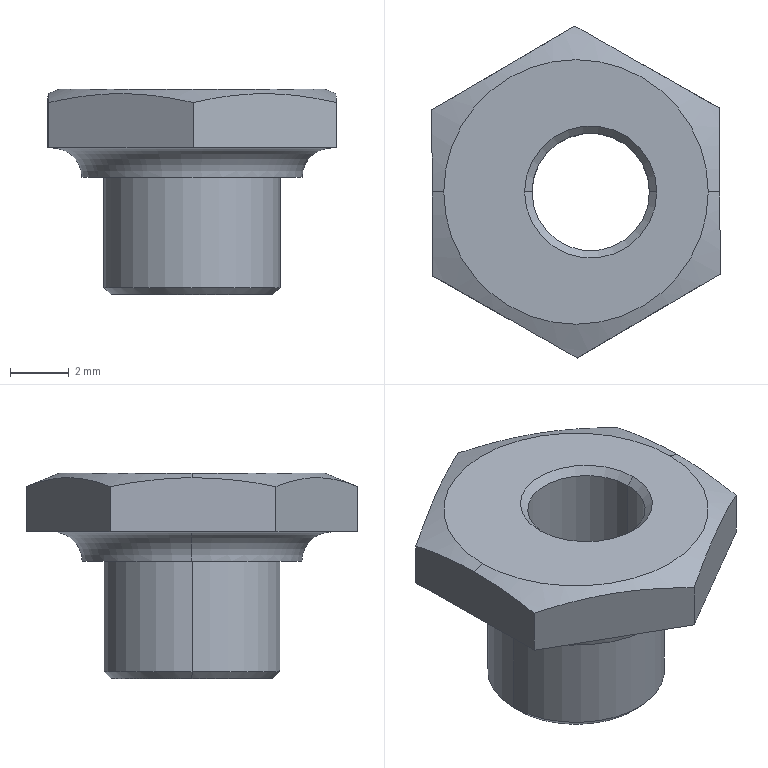Part | NX | features BREP 1 | 1 solid | 24 faces | box 9.818 x 11.293 x 7 mm | volume 236.126 mm3 | plane 10 | cone 8 | cylinder 4 | torus 2 | commonest cylinder face diameters 4 x2 6 x2
STEP:
#1=CARTESIAN_POINT('',(-3.,0.,0.25));
#2=VERTEX_POINT('',#1);
#3=CARTESIAN_POINT('',(-2.75,0.,0.));
#4=VERTEX_POINT('',#3);
#5=CARTESIAN_POINT('',(-3.,0.,0.25));
#6=DIRECTION('',(-0.7071,0.,0.7071));
#7=VECTOR('',#6,1000.);
#8=LINE('',#5,#7);
#9=EDGE_CURVE('',#2,#4,#8,.F.);
#10=ORIENTED_EDGE('',*,*,#9,.T.);
#11=CARTESIAN_POINT('',(2.75,0.,0.));
#12=VERTEX_POINT('',#11);
#13=CARTESIAN_POINT('',(0.,0.,0.));
#14=DIRECTION('',(0.,0.,-1.));
#15=DIRECTION('',(1.,0.,0.));
#16=AXIS2_PLACEMENT_3D('',#13,#14,#15);
#17=CIRCLE('',#16,2.75);
#18=EDGE_CURVE('',#12,#4,#17,.T.);
#19=ORIENTED_EDGE('',*,*,#18,.F.);
#20=CARTESIAN_POINT('',(3.,0.,0.25));
#21=VERTEX_POINT('',#20);
#22=CARTESIAN_POINT('',(3.,0.,0.25));
#23=DIRECTION('',(0.7071,0.,0.7071));
#24=VECTOR('',#23,1000.);
#25=LINE('',#22,#24);
#26=EDGE_CURVE('',#21,#12,#25,.F.);
#27=ORIENTED_EDGE('',*,*,#26,.F.);
#28=CARTESIAN_POINT('',(0.,0.,0.25));
#29=DIRECTION('',(0.,0.,1.));
#30=DIRECTION('',(1.,0.,0.));
#31=AXIS2_PLACEMENT_3D('',#28,#29,#30);
#32=CIRCLE('',#31,3.);
#33=EDGE_CURVE('',#2,#21,#32,.T.);
#34=ORIENTED_EDGE('',*,*,#33,.F.);
#35=EDGE_LOOP('',(#10,#19,#27,#34));
#36=FACE_BOUND('',#35,.T.);
#37=CARTESIAN_POINT('',(0.,0.,0.25));
#38=DIRECTION('',(0.,0.,1.));
#39=DIRECTION('',(1.,0.,0.));
#40=AXIS2_PLACEMENT_3D('',#37,#38,#39);
#41=CONICAL_SURFACE('',#40,3.,0.7854);
#42=ADVANCED_FACE('',(#36),#41,.T.);
#43=CARTESIAN_POINT('',(2.5,0.,0.25));
#44=VERTEX_POINT('',#43);
#45=CARTESIAN_POINT('',(2.75,0.,0.));
#46=DIRECTION('',(0.7071,0.,-0.7071));
#47=VECTOR('',#46,1000.);
#48=LINE('',#45,#47);
#49=EDGE_CURVE('',#44,#12,#48,.T.);
#50=ORIENTED_EDGE('',*,*,#49,.F.);
#51=CARTESIAN_POINT('',(-1.5,0.,0.25));
#52=VERTEX_POINT('',#51);
#53=CARTESIAN_POINT('',(0.5,0.,0.25));
#54=DIRECTION('',(0.,0.,-1.));
#55=DIRECTION('',(1.,0.,0.));
#56=AXIS2_PLACEMENT_3D('',#53,#54,#55);
#57=CIRCLE('',#56,2.);
#58=EDGE_CURVE('',#52,#44,#57,.T.);
#59=ORIENTED_EDGE('',*,*,#58,.F.);
#60=CARTESIAN_POINT('',(-1.75,0.,0.));
#61=VERTEX_POINT('',#60);
#62=CARTESIAN_POINT('',(-1.75,0.,0.));
#63=DIRECTION('',(-0.7071,0.,-0.7071));
#64=VECTOR('',#63,1000.);
#65=LINE('',#62,#64);
#66=EDGE_CURVE('',#52,#61,#65,.T.);
#67=ORIENTED_EDGE('',*,*,#66,.T.);
#68=CARTESIAN_POINT('',(0.5,0.,0.));
#69=DIRECTION('',(0.,0.,1.));
#70=DIRECTION('',(1.,0.,0.));
#71=AXIS2_PLACEMENT_3D('',#68,#69,#70);
#72=CIRCLE('',#71,2.25);
#73=EDGE_CURVE('',#12,#61,#72,.T.);
#74=ORIENTED_EDGE('',*,*,#73,.F.);
#75=EDGE_LOOP('',(#50,#59,#67,#74));
#76=FACE_BOUND('',#75,.T.);
#77=CARTESIAN_POINT('',(0.5,0.,0.));
#78=DIRECTION('',(0.,0.,-1.));
#79=DIRECTION('',(-1.,0.,0.));
#80=AXIS2_PLACEMENT_3D('',#77,#78,#79);
#81=CONICAL_SURFACE('',#80,2.25,0.7854);
#82=ADVANCED_FACE('',(#76),#81,.F.);
#83=CARTESIAN_POINT('',(-1.75,0.,7.));
#84=VERTEX_POINT('',#83);
#85=CARTESIAN_POINT('',(-1.5,0.,6.75));
#86=VERTEX_POINT('',#85);
#87=CARTESIAN_POINT('',(-1.5,0.,6.75));
#88=DIRECTION('',(-0.7071,0.,0.7071));
#89=VECTOR('',#88,1000.);
#90=LINE('',#87,#89);
#91=EDGE_CURVE('',#84,#86,#90,.F.);
#92=ORIENTED_EDGE('',*,*,#91,.T.);
#93=CARTESIAN_POINT('',(2.5,0.,6.75));
#94=VERTEX_POINT('',#93);
#95=CARTESIAN_POINT('',(0.5,0.,6.75));
#96=DIRECTION('',(0.,0.,1.));
#97=DIRECTION('',(1.,0.,0.));
#98=AXIS2_PLACEMENT_3D('',#95,#96,#97);
#99=CIRCLE('',#98,2.);
#100=EDGE_CURVE('',#94,#86,#99,.T.);
#101=ORIENTED_EDGE('',*,*,#100,.F.);
#102=CARTESIAN_POINT('',(2.75,0.,7.));
#103=VERTEX_POINT('',#102);
#104=CARTESIAN_POINT('',(2.5,0.,6.75));
#105=DIRECTION('',(0.7071,0.,0.7071));
#106=VECTOR('',#105,1000.);
#107=LINE('',#104,#106);
#108=EDGE_CURVE('',#103,#94,#107,.F.);
#109=ORIENTED_EDGE('',*,*,#108,.F.);
#110=CARTESIAN_POINT('',(0.5,0.,7.));
#111=DIRECTION('',(0.,0.,-1.));
#112=DIRECTION('',(1.,0.,0.));
#113=AXIS2_PLACEMENT_3D('',#110,#111,#112);
#114=CIRCLE('',#113,2.25);
#115=EDGE_CURVE('',#84,#103,#114,.T.);
#116=ORIENTED_EDGE('',*,*,#115,.F.);
#117=EDGE_LOOP('',(#92,#101,#109,#116));
#118=FACE_BOUND('',#117,.T.);
#119=CARTESIAN_POINT('',(0.5,0.,6.75));
#120=DIRECTION('',(0.,0.,1.));
#121=DIRECTION('',(1.,0.,0.));
#122=AXIS2_PLACEMENT_3D('',#119,#120,#121);
#123=CONICAL_SURFACE('',#122,2.,0.7854);
#124=ADVANCED_FACE('',(#118),#123,.F.);
#125=CARTESIAN_POINT('',(-3.75,0.,4.));
#126=VERTEX_POINT('',#125);
#127=CARTESIAN_POINT('',(-4.75,0.,5.));
#128=VERTEX_POINT('',#127);
#129=CARTESIAN_POINT('',(-4.75,0.,4.));
#130=DIRECTION('',(0.,1.,0.));
#131=DIRECTION('',(-1.,0.,0.));
#132=AXIS2_PLACEMENT_3D('',#129,#130,#131);
#133=CIRCLE('',#132,1.);
#134=EDGE_CURVE('',#126,#128,#133,.F.);
#135=ORIENTED_EDGE('',*,*,#134,.T.);
#136=CARTESIAN_POINT('',(4.75,0.,5.));
#137=VERTEX_POINT('',#136);
#138=CARTESIAN_POINT('',(0.,0.,5.));
#139=DIRECTION('',(0.,0.,1.));
#140=DIRECTION('',(1.,0.,0.));
#141=AXIS2_PLACEMENT_3D('',#138,#139,#140);
#142=CIRCLE('',#141,4.75);
#143=EDGE_CURVE('',#137,#128,#142,.T.);
#144=ORIENTED_EDGE('',*,*,#143,.F.);
#145=CARTESIAN_POINT('',(3.75,0.,4.));
#146=VERTEX_POINT('',#145);
#147=CARTESIAN_POINT('',(4.75,0.,4.));
#148=DIRECTION('',(0.,-1.,0.));
#149=DIRECTION('',(0.,0.,-1.));
#150=AXIS2_PLACEMENT_3D('',#147,#148,#149);
#151=CIRCLE('',#150,1.);
#152=EDGE_CURVE('',#146,#137,#151,.F.);
#153=ORIENTED_EDGE('',*,*,#152,.F.);
#154=CARTESIAN_POINT('',(0.,0.,4.));
#155=DIRECTION('',(0.,0.,-1.));
#156=DIRECTION('',(-1.,0.,0.));
#157=AXIS2_PLACEMENT_3D('',#154,#155,#156);
#158=CIRCLE('',#157,3.75);
#159=EDGE_CURVE('',#126,#146,#158,.T.);
#160=ORIENTED_EDGE('',*,*,#159,.F.);
#161=EDGE_LOOP('',(#135,#144,#153,#160));
#162=FACE_BOUND('',#161,.T.);
#163=CARTESIAN_POINT('',(0.,0.,4.));
#164=DIRECTION('',(0.,0.,1.));
#165=DIRECTION('',(1.,0.,0.));
#166=AXIS2_PLACEMENT_3D('',#163,#164,#165);
#167=TOROIDAL_SURFACE('',#166,4.75,1.);
#168=ADVANCED_FACE('',(#162),#167,.F.);
#169=CARTESIAN_POINT('',(-3.,0.,4.));
#170=VERTEX_POINT('',#169);
#171=CARTESIAN_POINT('',(3.,0.,4.));
#172=VERTEX_POINT('',#171);
#173=CARTESIAN_POINT('',(0.,0.,4.));
#174=DIRECTION('',(0.,0.,-1.));
#175=DIRECTION('',(-1.,0.,0.));
#176=AXIS2_PLACEMENT_3D('',#173,#174,#175);
#177=CIRCLE('',#176,3.);
#178=EDGE_CURVE('',#170,#172,#177,.T.);
#179=ORIENTED_EDGE('',*,*,#178,.F.);
#180=CARTESIAN_POINT('',(0.,0.,4.));
#181=DIRECTION('',(0.,0.,-1.));
#182=DIRECTION('',(-1.,0.,0.));
#183=AXIS2_PLACEMENT_3D('',#180,#181,#182);
#184=CIRCLE('',#183,3.);
#185=EDGE_CURVE('',#172,#170,#184,.T.);
#186=ORIENTED_EDGE('',*,*,#185,.F.);
#187=EDGE_LOOP('',(#179,#186));
#188=FACE_BOUND('',#187,.T.);
#189=CARTESIAN_POINT('',(0.,0.,4.));
#190=DIRECTION('',(0.,0.,-1.));
#191=DIRECTION('',(-1.,0.,0.));
#192=AXIS2_PLACEMENT_3D('',#189,#190,#191);
#193=CIRCLE('',#192,3.75);
#194=EDGE_CURVE('',#146,#126,#193,.T.);
#195=ORIENTED_EDGE('',*,*,#194,.T.);
#196=ORIENTED_EDGE('',*,*,#159,.T.);
#197=EDGE_LOOP('',(#195,#196));
#198=FACE_BOUND('',#197,.T.);
#199=CARTESIAN_POINT('',(0.,0.,4.));
#200=DIRECTION('',(0.,0.,-1.));
#201=DIRECTION('',(-1.,0.,0.));
#202=AXIS2_PLACEMENT_3D('',#199,#200,#201);
#203=PLANE('',#202);
#204=ADVANCED_FACE('',(#188,#198),#203,.T.);
#205=CARTESIAN_POINT('',(-4.909,2.79,5.));
#206=VERTEX_POINT('',#205);
#207=CARTESIAN_POINT('',(-4.909,2.79,6.541));
#208=VERTEX_POINT('',#207);
#209=CARTESIAN_POINT('',(-4.909,2.79,5.));
#210=DIRECTION('',(0.,0.,1.));
#211=VECTOR('',#210,1000.);
#212=LINE('',#209,#211);
#213=EDGE_CURVE('',#206,#208,#212,.T.);
#214=ORIENTED_EDGE('',*,*,#213,.F.);
#215=CARTESIAN_POINT('',(-4.871,-2.857,5.));
#216=VERTEX_POINT('',#215);
#217=CARTESIAN_POINT('',(-4.909,2.79,5.));
#218=DIRECTION('',(0.006849,-1.,0.));
#219=VECTOR('',#218,1000.);
#220=LINE('',#217,#219);
#221=EDGE_CURVE('',#206,#216,#220,.T.);
#222=ORIENTED_EDGE('',*,*,#221,.T.);
#223=CARTESIAN_POINT('',(-4.871,-2.857,6.541));
#224=VERTEX_POINT('',#223);
#225=CARTESIAN_POINT('',(-4.871,-2.857,5.));
#226=DIRECTION('',(0.,0.,1.));
#227=VECTOR('',#226,1000.);
#228=LINE('',#225,#227);
#229=EDGE_CURVE('',#216,#224,#228,.T.);
#230=ORIENTED_EDGE('',*,*,#229,.T.);
#231=CARTESIAN_POINT('',(-4.89,0.,6.844));
#232=VERTEX_POINT('',#231);
#233=CARTESIAN_POINT('',(-4.871,-2.857,6.541));
#234=CARTESIAN_POINT('',(-4.874,-2.356,6.642));
#235=CARTESIAN_POINT('',(-4.88,-1.445,6.789));
#236=CARTESIAN_POINT('',(-4.887,-0.467,6.845));
#237=CARTESIAN_POINT('',(-4.89,0.,6.844));
#238=B_SPLINE_CURVE_WITH_KNOTS('',3,(#233,#234,#235,#236,#237),.UNSPECIFIED.,.F.,.F.,(4,1,4),(0.,0.5,1.),.UNSPECIFIED.);
#239=EDGE_CURVE('',#232,#224,#238,.F.);
#240=ORIENTED_EDGE('',*,*,#239,.F.);
#241=CARTESIAN_POINT('',(-4.89,0.,6.844));
#242=CARTESIAN_POINT('',(-4.896,0.8631,6.842));
#243=CARTESIAN_POINT('',(-4.902,1.793,6.741));
#244=CARTESIAN_POINT('',(-4.909,2.79,6.541));
#245=B_SPLINE_CURVE_WITH_KNOTS('',3,(#241,#242,#243,#244),.UNSPECIFIED.,.F.,.F.,(4,4),(0.,1.),.UNSPECIFIED.);
#246=EDGE_CURVE('',#208,#232,#245,.F.);
#247=ORIENTED_EDGE('',*,*,#246,.F.);
#248=EDGE_LOOP('',(#214,#222,#230,#240,#247));
#249=FACE_BOUND('',#248,.T.);
#250=CARTESIAN_POINT('',(-4.909,2.79,5.));
#251=DIRECTION('',(-1.,-0.006849,0.));
#252=DIRECTION('',(0.006849,-1.,0.));
#253=AXIS2_PLACEMENT_3D('',#250,#251,#252);
#254=PLANE('',#253);
#255=ADVANCED_FACE('',(#249),#254,.T.);
#256=ORIENTED_EDGE('',*,*,#229,.F.);
#257=CARTESIAN_POINT('',(0.03867,-5.646,5.));
#258=VERTEX_POINT('',#257);
#259=CARTESIAN_POINT('',(-4.871,-2.857,5.));
#260=DIRECTION('',(0.8694,-0.4941,0.));
#261=VECTOR('',#260,1000.);
#262=LINE('',#259,#261);
#263=EDGE_CURVE('',#216,#258,#262,.T.);
#264=ORIENTED_EDGE('',*,*,#263,.T.);
#265=CARTESIAN_POINT('',(0.03867,-5.646,6.541));
#266=VERTEX_POINT('',#265);
#267=CARTESIAN_POINT('',(0.03867,-5.646,5.));
#268=DIRECTION('',(0.,0.,1.));
#269=VECTOR('',#268,1000.);
#270=LINE('',#267,#269);
#271=EDGE_CURVE('',#258,#266,#270,.T.);
#272=ORIENTED_EDGE('',*,*,#271,.T.);
#273=CARTESIAN_POINT('',(0.03867,-5.646,6.541));
#274=CARTESIAN_POINT('',(-1.719,-4.647,6.946));
#275=CARTESIAN_POINT('',(-3.121,-3.851,6.944));
#276=CARTESIAN_POINT('',(-4.871,-2.857,6.541));
#277=B_SPLINE_CURVE_WITH_KNOTS('',3,(#273,#274,#275,#276),.UNSPECIFIED.,.F.,.F.,(4,4),(0.,1.),.UNSPECIFIED.);
#278=EDGE_CURVE('',#224,#266,#277,.F.);
#279=ORIENTED_EDGE('',*,*,#278,.F.);
#280=EDGE_LOOP('',(#256,#264,#272,#279));
#281=FACE_BOUND('',#280,.T.);
#282=CARTESIAN_POINT('',(-4.871,-2.857,5.));
#283=DIRECTION('',(-0.4941,-0.8694,0.));
#284=DIRECTION('',(0.8694,-0.4941,0.));
#285=AXIS2_PLACEMENT_3D('',#282,#283,#284);
#286=PLANE('',#285);
#287=ADVANCED_FACE('',(#281),#286,.T.);
#288=ORIENTED_EDGE('',*,*,#271,.F.);
#289=CARTESIAN_POINT('',(4.909,-2.79,5.));
#290=VERTEX_POINT('',#289);
#291=CARTESIAN_POINT('',(0.03867,-5.646,5.));
#292=DIRECTION('',(0.8626,0.5059,0.));
#293=VECTOR('',#292,1000.);
#294=LINE('',#291,#293);
#295=EDGE_CURVE('',#258,#290,#294,.T.);
#296=ORIENTED_EDGE('',*,*,#295,.T.);
#297=CARTESIAN_POINT('',(4.909,-2.79,6.541));
#298=VERTEX_POINT('',#297);
#299=CARTESIAN_POINT('',(4.909,-2.79,5.));
#300=DIRECTION('',(0.,0.,1.));
#301=VECTOR('',#300,1000.);
#302=LINE('',#299,#301);
#303=EDGE_CURVE('',#290,#298,#302,.T.);
#304=ORIENTED_EDGE('',*,*,#303,.T.);
#305=CARTESIAN_POINT('',(4.909,-2.79,6.541));
#306=CARTESIAN_POINT('',(3.165,-3.813,6.946));
#307=CARTESIAN_POINT('',(1.775,-4.628,6.944));
#308=CARTESIAN_POINT('',(0.03867,-5.646,6.541));
#309=B_SPLINE_CURVE_WITH_KNOTS('',3,(#305,#306,#307,#308),.UNSPECIFIED.,.F.,.F.,(4,4),(0.,1.),.UNSPECIFIED.);
#310=EDGE_CURVE('',#266,#298,#309,.F.);
#311=ORIENTED_EDGE('',*,*,#310,.F.);
#312=EDGE_LOOP('',(#288,#296,#304,#311));
#313=FACE_BOUND('',#312,.T.);
#314=CARTESIAN_POINT('',(0.03867,-5.646,5.));
#315=DIRECTION('',(0.5059,-0.8626,0.));
#316=DIRECTION('',(0.8626,0.5059,0.));
#317=AXIS2_PLACEMENT_3D('',#314,#315,#316);
#318=PLANE('',#317);
#319=ADVANCED_FACE('',(#313),#318,.T.);
#320=ORIENTED_EDGE('',*,*,#303,.F.);
#321=CARTESIAN_POINT('',(4.871,2.857,5.));
#322=VERTEX_POINT('',#321);
#323=CARTESIAN_POINT('',(4.909,-2.79,5.));
#324=DIRECTION('',(-0.006849,1.,0.));
#325=VECTOR('',#324,1000.);
#326=LINE('',#323,#325);
#327=EDGE_CURVE('',#290,#322,#326,.T.);
#328=ORIENTED_EDGE('',*,*,#327,.T.);
#329=CARTESIAN_POINT('',(4.871,2.857,6.541));
#330=VERTEX_POINT('',#329);
#331=CARTESIAN_POINT('',(4.871,2.857,5.));
#332=DIRECTION('',(0.,0.,1.));
#333=VECTOR('',#332,1000.);
#334=LINE('',#331,#333);
#335=EDGE_CURVE('',#322,#330,#334,.T.);
#336=ORIENTED_EDGE('',*,*,#335,.T.);
#337=CARTESIAN_POINT('',(4.89,0.,6.844));
#338=VERTEX_POINT('',#337);
#339=CARTESIAN_POINT('',(4.871,2.857,6.541));
#340=CARTESIAN_POINT('',(4.874,2.356,6.642));
#341=CARTESIAN_POINT('',(4.88,1.445,6.789));
#342=CARTESIAN_POINT('',(4.887,0.467,6.845));
#343=CARTESIAN_POINT('',(4.89,0.,6.844));
#344=B_SPLINE_CURVE_WITH_KNOTS('',3,(#339,#340,#341,#342,#343),.UNSPECIFIED.,.F.,.F.,(4,1,4),(0.,0.5,1.),.UNSPECIFIED.);
#345=EDGE_CURVE('',#338,#330,#344,.F.);
#346=ORIENTED_EDGE('',*,*,#345,.F.);
#347=CARTESIAN_POINT('',(4.89,0.,6.844));
#348=CARTESIAN_POINT('',(4.896,-0.8631,6.842));
#349=CARTESIAN_POINT('',(4.902,-1.793,6.741));
#350=CARTESIAN_POINT('',(4.909,-2.79,6.541));
#351=B_SPLINE_CURVE_WITH_KNOTS('',3,(#347,#348,#349,#350),.UNSPECIFIED.,.F.,.F.,(4,4),(0.,1.),.UNSPECIFIED.);
#352=EDGE_CURVE('',#298,#338,#351,.F.);
#353=ORIENTED_EDGE('',*,*,#352,.F.);
#354=EDGE_LOOP('',(#320,#328,#336,#346,#353));
#355=FACE_BOUND('',#354,.T.);
#356=CARTESIAN_POINT('',(4.909,-2.79,5.));
#357=DIRECTION('',(1.,0.006849,0.));
#358=DIRECTION('',(-0.006849,1.,0.));
#359=AXIS2_PLACEMENT_3D('',#356,#357,#358);
#360=PLANE('',#359);
#361=ADVANCED_FACE('',(#355),#360,.T.);
#362=ORIENTED_EDGE('',*,*,#335,.F.);
#363=CARTESIAN_POINT('',(-0.03867,5.646,5.));
#364=VERTEX_POINT('',#363);
#365=CARTESIAN_POINT('',(4.871,2.857,5.));
#366=DIRECTION('',(-0.8694,0.4941,0.));
#367=VECTOR('',#366,1000.);
#368=LINE('',#365,#367);
#369=EDGE_CURVE('',#322,#364,#368,.T.);
#370=ORIENTED_EDGE('',*,*,#369,.T.);
#371=CARTESIAN_POINT('',(-0.03867,5.646,6.541));
#372=VERTEX_POINT('',#371);
#373=CARTESIAN_POINT('',(-0.03867,5.646,5.));
#374=DIRECTION('',(0.,0.,1.));
#375=VECTOR('',#374,1000.);
#376=LINE('',#373,#375);
#377=EDGE_CURVE('',#364,#372,#376,.T.);
#378=ORIENTED_EDGE('',*,*,#377,.T.);
#379=CARTESIAN_POINT('',(-0.03867,5.646,6.541));
#380=CARTESIAN_POINT('',(1.719,4.647,6.946));
#381=CARTESIAN_POINT('',(3.121,3.851,6.944));
#382=CARTESIAN_POINT('',(4.871,2.857,6.541));
#383=B_SPLINE_CURVE_WITH_KNOTS('',3,(#379,#380,#381,#382),.UNSPECIFIED.,.F.,.F.,(4,4),(0.,1.),.UNSPECIFIED.);
#384=EDGE_CURVE('',#330,#372,#383,.F.);
#385=ORIENTED_EDGE('',*,*,#384,.F.);
#386=EDGE_LOOP('',(#362,#370,#378,#385));
#387=FACE_BOUND('',#386,.T.);
#388=CARTESIAN_POINT('',(4.871,2.857,5.));
#389=DIRECTION('',(0.4941,0.8694,0.));
#390=DIRECTION('',(-0.8694,0.4941,0.));
#391=AXIS2_PLACEMENT_3D('',#388,#389,#390);
#392=PLANE('',#391);
#393=ADVANCED_FACE('',(#387),#392,.T.);
#394=ORIENTED_EDGE('',*,*,#377,.F.);
#395=CARTESIAN_POINT('',(-0.03867,5.646,5.));
#396=DIRECTION('',(-0.8626,-0.5059,0.));
#397=VECTOR('',#396,1000.);
#398=LINE('',#395,#397);
#399=EDGE_CURVE('',#364,#206,#398,.T.);
#400=ORIENTED_EDGE('',*,*,#399,.T.);
#401=ORIENTED_EDGE('',*,*,#213,.T.);
#402=CARTESIAN_POINT('',(-4.909,2.79,6.541));
#403=CARTESIAN_POINT('',(-3.165,3.813,6.946));
#404=CARTESIAN_POINT('',(-1.775,4.628,6.944));
#405=CARTESIAN_POINT('',(-0.03867,5.646,6.541));
#406=B_SPLINE_CURVE_WITH_KNOTS('',3,(#402,#403,#404,#405),.UNSPECIFIED.,.F.,.F.,(4,4),(0.,1.),.UNSPECIFIED.);
#407=EDGE_CURVE('',#372,#208,#406,.F.);
#408=ORIENTED_EDGE('',*,*,#407,.F.);
#409=EDGE_LOOP('',(#394,#400,#401,#408));
#410=FACE_BOUND('',#409,.T.);
#411=CARTESIAN_POINT('',(-0.03867,5.646,5.));
#412=DIRECTION('',(-0.5059,0.8626,0.));
#413=DIRECTION('',(-0.8626,-0.5059,0.));
#414=AXIS2_PLACEMENT_3D('',#411,#412,#413);
#415=PLANE('',#414);
#416=ADVANCED_FACE('',(#410),#415,.T.);
#417=CARTESIAN_POINT('',(2.5,0.,7.));
#418=DIRECTION('',(0.,0.,-1.));
#419=VECTOR('',#418,1000.);
#420=LINE('',#417,#419);
#421=EDGE_CURVE('',#94,#44,#420,.T.);
#422=ORIENTED_EDGE('',*,*,#421,.F.);
#423=ORIENTED_EDGE('',*,*,#100,.T.);
#424=CARTESIAN_POINT('',(-1.5,0.,7.));
#425=DIRECTION('',(0.,0.,-1.));
#426=VECTOR('',#425,1000.);
#427=LINE('',#424,#426);
#428=EDGE_CURVE('',#86,#52,#427,.T.);
#429=ORIENTED_EDGE('',*,*,#428,.T.);
#430=ORIENTED_EDGE('',*,*,#58,.T.);
#431=EDGE_LOOP('',(#422,#423,#429,#430));
#432=FACE_BOUND('',#431,.T.);
#433=CARTESIAN_POINT('',(0.5,0.,7.));
#434=DIRECTION('',(0.,0.,-1.));
#435=DIRECTION('',(-1.,0.,0.));
#436=AXIS2_PLACEMENT_3D('',#433,#434,#435);
#437=CYLINDRICAL_SURFACE('',#436,2.);
#438=ADVANCED_FACE('',(#432),#437,.F.);
#439=ORIENTED_EDGE('',*,*,#18,.T.);
#440=CARTESIAN_POINT('',(0.,0.,0.));
#441=DIRECTION('',(0.,0.,-1.));
#442=DIRECTION('',(1.,0.,0.));
#443=AXIS2_PLACEMENT_3D('',#440,#441,#442);
#444=CIRCLE('',#443,2.75);
#445=EDGE_CURVE('',#4,#12,#444,.T.);
#446=ORIENTED_EDGE('',*,*,#445,.T.);
#447=ORIENTED_EDGE('',*,*,#73,.T.);
#448=CARTESIAN_POINT('',(0.5,0.,0.));
#449=DIRECTION('',(0.,0.,1.));
#450=DIRECTION('',(1.,0.,0.));
#451=AXIS2_PLACEMENT_3D('',#448,#449,#450);
#452=CIRCLE('',#451,2.25);
#453=EDGE_CURVE('',#61,#12,#452,.T.);
#454=ORIENTED_EDGE('',*,*,#453,.T.);
#455=EDGE_LOOP('',(#439,#446,#447,#454));
#456=FACE_BOUND('',#455,.T.);
#457=CARTESIAN_POINT('',(0.,0.,0.));
#458=DIRECTION('',(0.,0.,1.));
#459=DIRECTION('',(1.,0.,0.));
#460=AXIS2_PLACEMENT_3D('',#457,#458,#459);
#461=PLANE('',#460);
#462=ADVANCED_FACE('',(#456),#461,.F.);
#463=CARTESIAN_POINT('',(-4.5,0.,7.));
#464=VERTEX_POINT('',#463);
#465=CARTESIAN_POINT('',(4.5,0.,7.));
#466=VERTEX_POINT('',#465);
#467=CARTESIAN_POINT('',(0.,0.,7.));
#468=DIRECTION('',(0.,0.,1.));
#469=DIRECTION('',(1.,0.,0.));
#470=AXIS2_PLACEMENT_3D('',#467,#468,#469);
#471=CIRCLE('',#470,4.5);
#472=EDGE_CURVE('',#464,#466,#471,.T.);
#473=ORIENTED_EDGE('',*,*,#472,.T.);
#474=CARTESIAN_POINT('',(0.,0.,7.));
#475=DIRECTION('',(0.,0.,1.));
#476=DIRECTION('',(1.,0.,0.));
#477=AXIS2_PLACEMENT_3D('',#474,#475,#476);
#478=CIRCLE('',#477,4.5);
#479=EDGE_CURVE('',#466,#464,#478,.T.);
#480=ORIENTED_EDGE('',*,*,#479,.T.);
#481=EDGE_LOOP('',(#473,#480));
#482=FACE_BOUND('',#481,.T.);
#483=CARTESIAN_POINT('',(0.5,0.,7.));
#484=DIRECTION('',(0.,0.,-1.));
#485=DIRECTION('',(1.,0.,0.));
#486=AXIS2_PLACEMENT_3D('',#483,#484,#485);
#487=CIRCLE('',#486,2.25);
#488=EDGE_CURVE('',#103,#84,#487,.T.);
#489=ORIENTED_EDGE('',*,*,#488,.T.);
#490=ORIENTED_EDGE('',*,*,#115,.T.);
#491=EDGE_LOOP('',(#489,#490));
#492=FACE_BOUND('',#491,.T.);
#493=CARTESIAN_POINT('',(0.,0.,7.));
#494=DIRECTION('',(0.,0.,1.));
#495=DIRECTION('',(1.,0.,0.));
#496=AXIS2_PLACEMENT_3D('',#493,#494,#495);
#497=PLANE('',#496);
#498=ADVANCED_FACE('',(#482,#492),#497,.T.);
#499=CARTESIAN_POINT('',(3.,0.,7.));
#500=DIRECTION('',(0.,0.,-1.));
#501=VECTOR('',#500,1000.);
#502=LINE('',#499,#501);
#503=EDGE_CURVE('',#172,#21,#502,.T.);
#504=ORIENTED_EDGE('',*,*,#503,.F.);
#505=ORIENTED_EDGE('',*,*,#185,.T.);
#506=CARTESIAN_POINT('',(-3.,0.,7.));
#507=DIRECTION('',(0.,0.,-1.));
#508=VECTOR('',#507,1000.);
#509=LINE('',#506,#508);
#510=EDGE_CURVE('',#170,#2,#509,.T.);
#511=ORIENTED_EDGE('',*,*,#510,.T.);
#512=ORIENTED_EDGE('',*,*,#33,.T.);
#513=EDGE_LOOP('',(#504,#505,#511,#512));
#514=FACE_BOUND('',#513,.T.);
#515=CARTESIAN_POINT('',(0.,0.,7.));
#516=DIRECTION('',(0.,0.,-1.));
#517=DIRECTION('',(-1.,0.,0.));
#518=AXIS2_PLACEMENT_3D('',#515,#516,#517);
#519=CYLINDRICAL_SURFACE('',#518,3.);
#520=ADVANCED_FACE('',(#514),#519,.T.);
#521=CARTESIAN_POINT('',(4.5,0.,7.));
#522=DIRECTION('',(0.9285,0.,-0.3714));
#523=VECTOR('',#522,1000.);
#524=LINE('',#521,#523);
#525=EDGE_CURVE('',#466,#338,#524,.T.);
#526=ORIENTED_EDGE('',*,*,#525,.F.);
#527=ORIENTED_EDGE('',*,*,#472,.F.);
#528=CARTESIAN_POINT('',(-4.5,0.,7.));
#529=DIRECTION('',(-0.9285,0.,-0.3714));
#530=VECTOR('',#529,1000.);
#531=LINE('',#528,#530);
#532=EDGE_CURVE('',#464,#232,#531,.T.);
#533=ORIENTED_EDGE('',*,*,#532,.T.);
#534=ORIENTED_EDGE('',*,*,#239,.T.);
#535=ORIENTED_EDGE('',*,*,#278,.T.);
#536=ORIENTED_EDGE('',*,*,#310,.T.);
#537=ORIENTED_EDGE('',*,*,#352,.T.);
#538=EDGE_LOOP('',(#526,#527,#533,#534,#535,#536,#537));
#539=FACE_BOUND('',#538,.T.);
#540=CARTESIAN_POINT('',(0.,0.,7.));
#541=DIRECTION('',(0.,0.,-1.));
#542=DIRECTION('',(-1.,0.,0.));
#543=AXIS2_PLACEMENT_3D('',#540,#541,#542);
#544=CONICAL_SURFACE('',#543,4.5,1.19);
#545=ADVANCED_FACE('',(#539),#544,.T.);
#546=ORIENTED_EDGE('',*,*,#399,.F.);
#547=ORIENTED_EDGE('',*,*,#369,.F.);
#548=ORIENTED_EDGE('',*,*,#327,.F.);
#549=ORIENTED_EDGE('',*,*,#295,.F.);
#550=ORIENTED_EDGE('',*,*,#263,.F.);
#551=ORIENTED_EDGE('',*,*,#221,.F.);
#552=EDGE_LOOP('',(#546,#547,#548,#549,#550,#551));
#553=FACE_BOUND('',#552,.T.);
#554=ORIENTED_EDGE('',*,*,#143,.T.);
#555=CARTESIAN_POINT('',(0.,0.,5.));
#556=DIRECTION('',(0.,0.,1.));
#557=DIRECTION('',(1.,0.,0.));
#558=AXIS2_PLACEMENT_3D('',#555,#556,#557);
#559=CIRCLE('',#558,4.75);
#560=EDGE_CURVE('',#128,#137,#559,.T.);
#561=ORIENTED_EDGE('',*,*,#560,.T.);
#562=EDGE_LOOP('',(#554,#561));
#563=FACE_BOUND('',#562,.T.);
#564=CARTESIAN_POINT('',(0.,0.,5.));
#565=DIRECTION('',(0.,0.,1.));
#566=DIRECTION('',(1.,0.,0.));
#567=AXIS2_PLACEMENT_3D('',#564,#565,#566);
#568=PLANE('',#567);
#569=ADVANCED_FACE('',(#553,#563),#568,.F.);
#570=ORIENTED_EDGE('',*,*,#479,.F.);
#571=ORIENTED_EDGE('',*,*,#525,.T.);
#572=ORIENTED_EDGE('',*,*,#345,.T.);
#573=ORIENTED_EDGE('',*,*,#384,.T.);
#574=ORIENTED_EDGE('',*,*,#407,.T.);
#575=ORIENTED_EDGE('',*,*,#246,.T.);
#576=ORIENTED_EDGE('',*,*,#532,.F.);
#577=EDGE_LOOP('',(#570,#571,#572,#573,#574,#575,#576));
#578=FACE_BOUND('',#577,.T.);
#579=CARTESIAN_POINT('',(0.,0.,7.));
#580=DIRECTION('',(0.,0.,-1.));
#581=DIRECTION('',(-1.,0.,0.));
#582=AXIS2_PLACEMENT_3D('',#579,#580,#581);
#583=CONICAL_SURFACE('',#582,4.5,1.19);
#584=ADVANCED_FACE('',(#578),#583,.T.);
#585=ORIENTED_EDGE('',*,*,#178,.T.);
#586=ORIENTED_EDGE('',*,*,#503,.T.);
#587=CARTESIAN_POINT('',(0.,0.,0.25));
#588=DIRECTION('',(0.,0.,1.));
#589=DIRECTION('',(1.,0.,0.));
#590=AXIS2_PLACEMENT_3D('',#587,#588,#589);
#591=CIRCLE('',#590,3.);
#592=EDGE_CURVE('',#21,#2,#591,.T.);
#593=ORIENTED_EDGE('',*,*,#592,.T.);
#594=ORIENTED_EDGE('',*,*,#510,.F.);
#595=EDGE_LOOP('',(#585,#586,#593,#594));
#596=FACE_BOUND('',#595,.T.);
#597=CARTESIAN_POINT('',(0.,0.,7.));
#598=DIRECTION('',(0.,0.,-1.));
#599=DIRECTION('',(-1.,0.,0.));
#600=AXIS2_PLACEMENT_3D('',#597,#598,#599);
#601=CYLINDRICAL_SURFACE('',#600,3.);
#602=ADVANCED_FACE('',(#596),#601,.T.);
#603=CARTESIAN_POINT('',(0.5,0.,6.75));
#604=DIRECTION('',(0.,0.,1.));
#605=DIRECTION('',(1.,0.,0.));
#606=AXIS2_PLACEMENT_3D('',#603,#604,#605);
#607=CIRCLE('',#606,2.);
#608=EDGE_CURVE('',#86,#94,#607,.T.);
#609=ORIENTED_EDGE('',*,*,#608,.T.);
#610=ORIENTED_EDGE('',*,*,#421,.T.);
#611=CARTESIAN_POINT('',(0.5,0.,0.25));
#612=DIRECTION('',(0.,0.,-1.));
#613=DIRECTION('',(1.,0.,0.));
#614=AXIS2_PLACEMENT_3D('',#611,#612,#613);
#615=CIRCLE('',#614,2.);
#616=EDGE_CURVE('',#44,#52,#615,.T.);
#617=ORIENTED_EDGE('',*,*,#616,.T.);
#618=ORIENTED_EDGE('',*,*,#428,.F.);
#619=EDGE_LOOP('',(#609,#610,#617,#618));
#620=FACE_BOUND('',#619,.T.);
#621=CARTESIAN_POINT('',(0.5,0.,7.));
#622=DIRECTION('',(0.,0.,-1.));
#623=DIRECTION('',(-1.,0.,0.));
#624=AXIS2_PLACEMENT_3D('',#621,#622,#623);
#625=CYLINDRICAL_SURFACE('',#624,2.);
#626=ADVANCED_FACE('',(#620),#625,.F.);
#627=ORIENTED_EDGE('',*,*,#560,.F.);
#628=ORIENTED_EDGE('',*,*,#134,.F.);
#629=ORIENTED_EDGE('',*,*,#194,.F.);
#630=ORIENTED_EDGE('',*,*,#152,.T.);
#631=EDGE_LOOP('',(#627,#628,#629,#630));
#632=FACE_BOUND('',#631,.T.);
#633=CARTESIAN_POINT('',(0.,0.,4.));
#634=DIRECTION('',(0.,0.,1.));
#635=DIRECTION('',(1.,0.,0.));
#636=AXIS2_PLACEMENT_3D('',#633,#634,#635);
#637=TOROIDAL_SURFACE('',#636,4.75,1.);
#638=ADVANCED_FACE('',(#632),#637,.F.);
#639=ORIENTED_EDGE('',*,*,#608,.F.);
#640=ORIENTED_EDGE('',*,*,#91,.F.);
#641=ORIENTED_EDGE('',*,*,#488,.F.);
#642=ORIENTED_EDGE('',*,*,#108,.T.);
#643=EDGE_LOOP('',(#639,#640,#641,#642));
#644=FACE_BOUND('',#643,.T.);
#645=CARTESIAN_POINT('',(0.5,0.,6.75));
#646=DIRECTION('',(0.,0.,1.));
#647=DIRECTION('',(1.,0.,0.));
#648=AXIS2_PLACEMENT_3D('',#645,#646,#647);
#649=CONICAL_SURFACE('',#648,2.,0.7854);
#650=ADVANCED_FACE('',(#644),#649,.F.);
#651=ORIENTED_EDGE('',*,*,#616,.F.);
#652=ORIENTED_EDGE('',*,*,#49,.T.);
#653=ORIENTED_EDGE('',*,*,#453,.F.);
#654=ORIENTED_EDGE('',*,*,#66,.F.);
#655=EDGE_LOOP('',(#651,#652,#653,#654));
#656=FACE_BOUND('',#655,.T.);
#657=CARTESIAN_POINT('',(0.5,0.,0.));
#658=DIRECTION('',(0.,0.,-1.));
#659=DIRECTION('',(-1.,0.,0.));
#660=AXIS2_PLACEMENT_3D('',#657,#658,#659);
#661=CONICAL_SURFACE('',#660,2.25,0.7854);
#662=ADVANCED_FACE('',(#656),#661,.F.);
#663=ORIENTED_EDGE('',*,*,#445,.F.);
#664=ORIENTED_EDGE('',*,*,#9,.F.);
#665=ORIENTED_EDGE('',*,*,#592,.F.);
#666=ORIENTED_EDGE('',*,*,#26,.T.);
#667=EDGE_LOOP('',(#663,#664,#665,#666));
#668=FACE_BOUND('',#667,.T.);
#669=CARTESIAN_POINT('',(0.,0.,0.25));
#670=DIRECTION('',(0.,0.,1.));
#671=DIRECTION('',(1.,0.,0.));
#672=AXIS2_PLACEMENT_3D('',#669,#670,#671);
#673=CONICAL_SURFACE('',#672,3.,0.7854);
#674=ADVANCED_FACE('',(#668),#673,.T.);
#675=CLOSED_SHELL('',(#42,#82,#124,#168,#204,#255,#287,#319,#361,#393,#416,#438,#462,#498,#520,#545,#569,#584,#602,#626,#638,#650,#662,#674));
#676=MANIFOLD_SOLID_BREP('',#675);
#677=(LENGTH_UNIT()NAMED_UNIT(*)SI_UNIT(.MILLI.,.METRE.));
#678=UNCERTAINTY_MEASURE_WITH_UNIT(LENGTH_MEASURE(0.0508),#677,'','');
#679=(NAMED_UNIT(*)PLANE_ANGLE_UNIT()SI_UNIT($,.RADIAN.));
#680=(NAMED_UNIT(*)SI_UNIT($,.STERADIAN.)SOLID_ANGLE_UNIT());
#681=(GEOMETRIC_REPRESENTATION_CONTEXT(3)GLOBAL_UNCERTAINTY_ASSIGNED_CONTEXT((#678))GLOBAL_UNIT_ASSIGNED_CONTEXT((#677,#679,#680))REPRESENTATION_CONTEXT('',''));
#682=ADVANCED_BREP_SHAPE_REPRESENTATION('',(#676),#681);